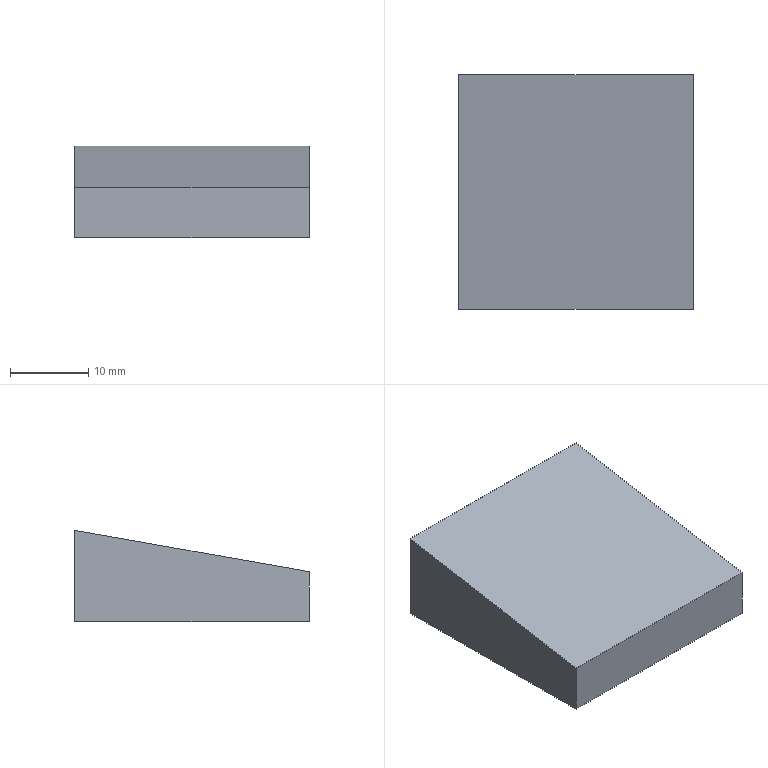Part | NX | features solid 2 | 1 solid | 6 faces | box 30 x 30 x 11.676 mm | volume 8128 mm3 | plane 6
STEP:
#1=CARTESIAN_POINT('',(205.,-165.,-50.));
#2=VERTEX_POINT('',#1);
#3=CARTESIAN_POINT('',(205.,-195.,-50.));
#4=VERTEX_POINT('',#3);
#5=CARTESIAN_POINT('',(205.,-195.,-50.));
#6=DIRECTION('',(0.,-1.,0.));
#7=VECTOR('',#6,1000.);
#8=LINE('',#5,#7);
#9=EDGE_CURVE('',#2,#4,#8,.T.);
#10=ORIENTED_EDGE('',*,*,#9,.F.);
#11=CARTESIAN_POINT('',(205.,-165.,-38.324));
#12=VERTEX_POINT('',#11);
#13=CARTESIAN_POINT('',(205.,-165.,-110.));
#14=DIRECTION('',(0.,0.,1.));
#15=VECTOR('',#14,1000.);
#16=LINE('',#13,#15);
#17=EDGE_CURVE('',#2,#12,#16,.T.);
#18=ORIENTED_EDGE('',*,*,#17,.T.);
#19=CARTESIAN_POINT('',(205.,-195.,-43.614));
#20=VERTEX_POINT('',#19);
#21=CARTESIAN_POINT('',(205.,-196.092,-43.807));
#22=DIRECTION('',(0.,0.9848,0.1736));
#23=VECTOR('',#22,1000.);
#24=LINE('',#21,#23);
#25=EDGE_CURVE('',#20,#12,#24,.T.);
#26=ORIENTED_EDGE('',*,*,#25,.F.);
#27=CARTESIAN_POINT('',(205.,-195.,-110.));
#28=DIRECTION('',(0.,0.,1.));
#29=VECTOR('',#28,1000.);
#30=LINE('',#27,#29);
#31=EDGE_CURVE('',#4,#20,#30,.T.);
#32=ORIENTED_EDGE('',*,*,#31,.F.);
#33=EDGE_LOOP('',(#10,#18,#26,#32));
#34=FACE_BOUND('',#33,.T.);
#35=CARTESIAN_POINT('',(205.,-195.,-110.));
#36=DIRECTION('',(-1.,0.,0.));
#37=DIRECTION('',(0.,0.,-1.));
#38=AXIS2_PLACEMENT_3D('',#35,#36,#37);
#39=PLANE('',#38);
#40=ADVANCED_FACE('',(#34),#39,.F.);
#41=CARTESIAN_POINT('',(175.,-195.,-50.));
#42=VERTEX_POINT('',#41);
#43=CARTESIAN_POINT('',(175.,-195.,-43.614));
#44=VERTEX_POINT('',#43);
#45=CARTESIAN_POINT('',(175.,-195.,-110.));
#46=DIRECTION('',(0.,0.,1.));
#47=VECTOR('',#46,1000.);
#48=LINE('',#45,#47);
#49=EDGE_CURVE('',#42,#44,#48,.T.);
#50=ORIENTED_EDGE('',*,*,#49,.F.);
#51=CARTESIAN_POINT('',(205.,-195.,-50.));
#52=DIRECTION('',(1.,0.,0.));
#53=VECTOR('',#52,1000.);
#54=LINE('',#51,#53);
#55=EDGE_CURVE('',#42,#4,#54,.T.);
#56=ORIENTED_EDGE('',*,*,#55,.T.);
#57=ORIENTED_EDGE('',*,*,#31,.T.);
#58=CARTESIAN_POINT('',(215.,-195.,-43.614));
#59=DIRECTION('',(1.,0.,0.));
#60=VECTOR('',#59,1000.);
#61=LINE('',#58,#60);
#62=EDGE_CURVE('',#20,#44,#61,.F.);
#63=ORIENTED_EDGE('',*,*,#62,.T.);
#64=EDGE_LOOP('',(#50,#56,#57,#63));
#65=FACE_BOUND('',#64,.T.);
#66=CARTESIAN_POINT('',(205.,-195.,-110.));
#67=DIRECTION('',(0.,-1.,0.));
#68=DIRECTION('',(0.,0.,-1.));
#69=AXIS2_PLACEMENT_3D('',#66,#67,#68);
#70=PLANE('',#69);
#71=ADVANCED_FACE('',(#65),#70,.T.);
#72=CARTESIAN_POINT('',(175.,-165.,-50.));
#73=VERTEX_POINT('',#72);
#74=CARTESIAN_POINT('',(175.,-165.,-38.324));
#75=VERTEX_POINT('',#74);
#76=CARTESIAN_POINT('',(175.,-165.,-110.));
#77=DIRECTION('',(0.,0.,1.));
#78=VECTOR('',#77,1000.);
#79=LINE('',#76,#78);
#80=EDGE_CURVE('',#73,#75,#79,.T.);
#81=ORIENTED_EDGE('',*,*,#80,.F.);
#82=CARTESIAN_POINT('',(175.,-195.,-50.));
#83=DIRECTION('',(0.,-1.,0.));
#84=VECTOR('',#83,1000.);
#85=LINE('',#82,#84);
#86=EDGE_CURVE('',#73,#42,#85,.T.);
#87=ORIENTED_EDGE('',*,*,#86,.T.);
#88=ORIENTED_EDGE('',*,*,#49,.T.);
#89=CARTESIAN_POINT('',(175.,-165.,-38.324));
#90=DIRECTION('',(0.,-0.9848,-0.1736));
#91=VECTOR('',#90,1000.);
#92=LINE('',#89,#91);
#93=EDGE_CURVE('',#44,#75,#92,.F.);
#94=ORIENTED_EDGE('',*,*,#93,.T.);
#95=EDGE_LOOP('',(#81,#87,#88,#94));
#96=FACE_BOUND('',#95,.T.);
#97=CARTESIAN_POINT('',(175.,-195.,-110.));
#98=DIRECTION('',(-1.,0.,0.));
#99=DIRECTION('',(0.,0.,-1.));
#100=AXIS2_PLACEMENT_3D('',#97,#98,#99);
#101=PLANE('',#100);
#102=ADVANCED_FACE('',(#96),#101,.T.);
#103=CARTESIAN_POINT('',(205.,-165.,-50.));
#104=DIRECTION('',(1.,0.,0.));
#105=VECTOR('',#104,1000.);
#106=LINE('',#103,#105);
#107=EDGE_CURVE('',#73,#2,#106,.T.);
#108=ORIENTED_EDGE('',*,*,#107,.F.);
#109=ORIENTED_EDGE('',*,*,#80,.T.);
#110=CARTESIAN_POINT('',(205.,-165.,-38.324));
#111=DIRECTION('',(-1.,0.,0.));
#112=VECTOR('',#111,1000.);
#113=LINE('',#110,#112);
#114=EDGE_CURVE('',#12,#75,#113,.T.);
#115=ORIENTED_EDGE('',*,*,#114,.F.);
#116=ORIENTED_EDGE('',*,*,#17,.F.);
#117=EDGE_LOOP('',(#108,#109,#115,#116));
#118=FACE_BOUND('',#117,.T.);
#119=CARTESIAN_POINT('',(205.,-165.,-110.));
#120=DIRECTION('',(0.,-1.,0.));
#121=DIRECTION('',(0.,0.,-1.));
#122=AXIS2_PLACEMENT_3D('',#119,#120,#121);
#123=PLANE('',#122);
#124=ADVANCED_FACE('',(#118),#123,.F.);
#125=ORIENTED_EDGE('',*,*,#114,.T.);
#126=ORIENTED_EDGE('',*,*,#93,.F.);
#127=ORIENTED_EDGE('',*,*,#62,.F.);
#128=ORIENTED_EDGE('',*,*,#25,.T.);
#129=EDGE_LOOP('',(#125,#126,#127,#128));
#130=FACE_BOUND('',#129,.T.);
#131=CARTESIAN_POINT('',(215.,-165.,-38.324));
#132=DIRECTION('',(0.,0.1736,-0.9848));
#133=DIRECTION('',(0.,0.9848,0.1736));
#134=AXIS2_PLACEMENT_3D('',#131,#132,#133);
#135=PLANE('',#134);
#136=ADVANCED_FACE('',(#130),#135,.F.);
#137=ORIENTED_EDGE('',*,*,#86,.F.);
#138=ORIENTED_EDGE('',*,*,#107,.T.);
#139=ORIENTED_EDGE('',*,*,#9,.T.);
#140=ORIENTED_EDGE('',*,*,#55,.F.);
#141=EDGE_LOOP('',(#137,#138,#139,#140));
#142=FACE_BOUND('',#141,.T.);
#143=CARTESIAN_POINT('',(-140.,-165.,-50.));
#144=DIRECTION('',(0.,0.,-1.));
#145=DIRECTION('',(-1.,0.,0.));
#146=AXIS2_PLACEMENT_3D('',#143,#144,#145);
#147=PLANE('',#146);
#148=ADVANCED_FACE('',(#142),#147,.T.);
#149=CLOSED_SHELL('',(#40,#71,#102,#124,#136,#148));
#150=MANIFOLD_SOLID_BREP('',#149);
#151=(LENGTH_UNIT()NAMED_UNIT(*)SI_UNIT(.MILLI.,.METRE.));
#152=UNCERTAINTY_MEASURE_WITH_UNIT(LENGTH_MEASURE(0.00001),#151,'','');
#153=(NAMED_UNIT(*)PLANE_ANGLE_UNIT()SI_UNIT($,.RADIAN.));
#154=(NAMED_UNIT(*)SI_UNIT($,.STERADIAN.)SOLID_ANGLE_UNIT());
#155=(GEOMETRIC_REPRESENTATION_CONTEXT(3)GLOBAL_UNCERTAINTY_ASSIGNED_CONTEXT((#152))GLOBAL_UNIT_ASSIGNED_CONTEXT((#151,#153,#154))REPRESENTATION_CONTEXT('',''));
#156=ADVANCED_BREP_SHAPE_REPRESENTATION('',(#150),#155);